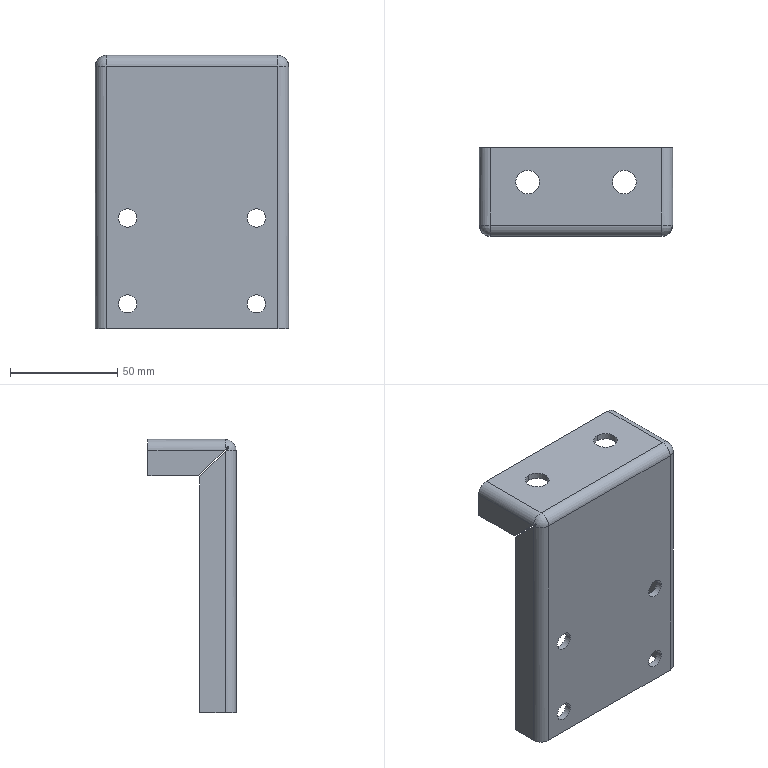Part | SolidWorks | features BaseBody 1 | 1 solid | 46 faces | box 90 x 41 x 127.2 mm | volume 53821 mm3 | cylinder 22 | plane 22 | sphere 2 | commonest cylinder face diameters 8.5 x8 4 x5 10 x5 11 x4